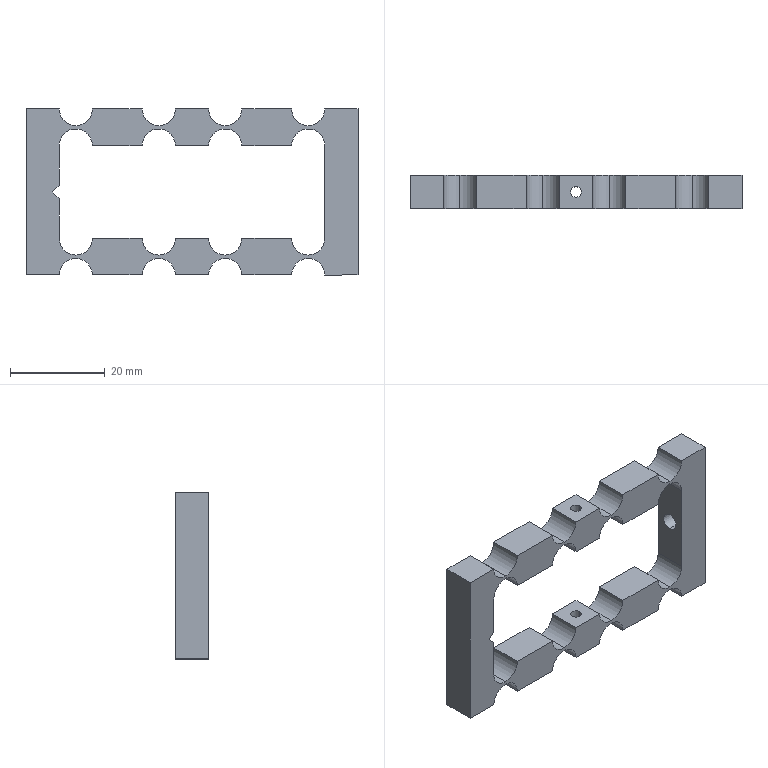Part | SolidWorks | features Extrusion 1, HoleWzd 1, ICE 1, Scale 1 | 1 solid | 55 faces | box 70 x 7 x 35 mm | volume 7163 mm3 | cylinder 30 | plane 25 | commonest cylinder face diameters 7 x24 2.31 x4 3.57 x2